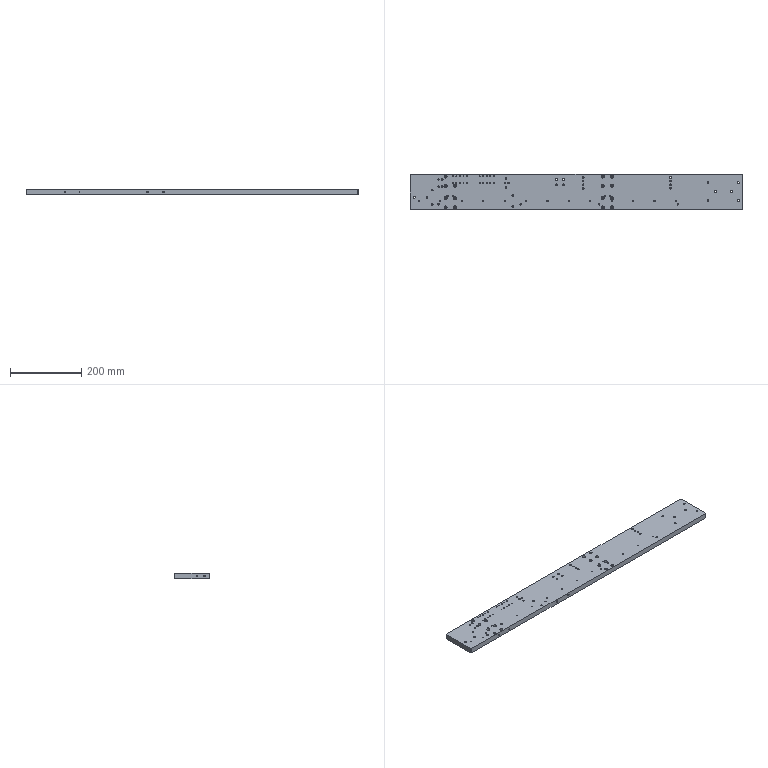Part | SolidWorks | features HoleWzd 10, Chamfer 1, Extrusion 1, LPattern 1 | 1 solid | 349 faces | box 930 x 100 x 15 mm | volume 1375215 mm3 | cylinder 232 | cone 92 | plane 25 | commonest cylinder face diameters 2.5 x44 3.3 x44 5 x44 4 x36 4.5 x30 8 x30